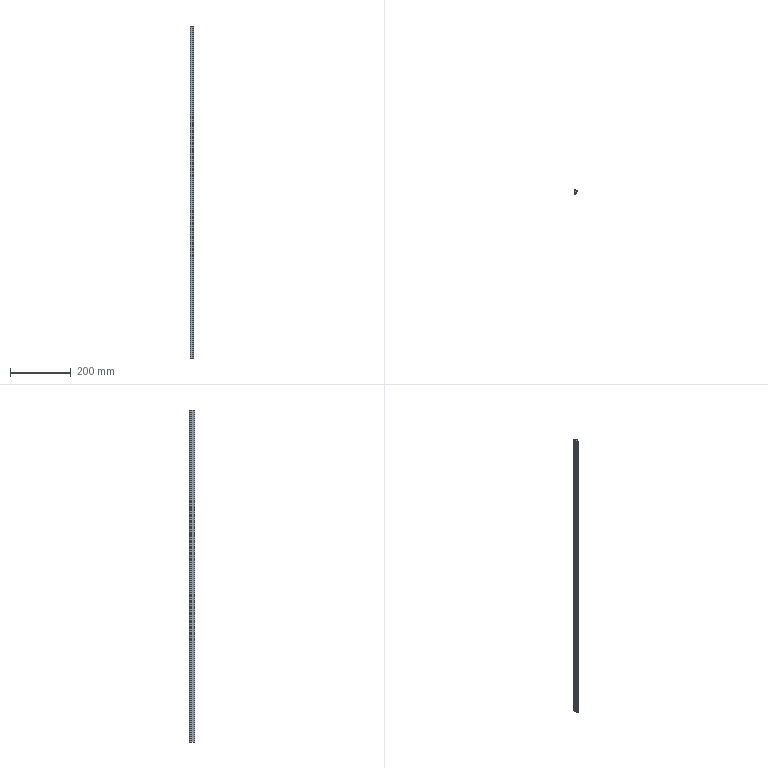Part | SolidWorks | features BaseBody 1, MoveFace 1 | 1 solid | 20 faces | box 10.8 x 17.5 x 1090 mm | volume 85893 mm3 | cylinder 11 | plane 9 | commonest cylinder face diameters 1.6 x2 14 x2 0.4 x1 0.6 x1 0.8 x1 2.6 x1
STEP:
#1=CARTESIAN_POINT('',(-3.236,-11.055,990.));
#2=VERTEX_POINT('',#1);
#3=CARTESIAN_POINT('',(-4.3,-10.3,990.));
#4=VERTEX_POINT('',#3);
#5=CARTESIAN_POINT('',(-3.5,-10.3,990.));
#6=DIRECTION('',(0.,0.,-1.));
#7=DIRECTION('',(1.,0.,0.));
#8=AXIS2_PLACEMENT_3D('',#5,#6,#7);
#9=CIRCLE('',#8,0.8);
#10=EDGE_CURVE('',#2,#4,#9,.T.);
#11=ORIENTED_EDGE('',*,*,#10,.T.);
#12=CARTESIAN_POINT('',(-4.3,-10.3,-100.));
#13=VERTEX_POINT('',#12);
#14=CARTESIAN_POINT('',(-4.3,-10.3,-100.));
#15=DIRECTION('',(0.,0.,-1.));
#16=VECTOR('',#15,1000.);
#17=LINE('',#14,#16);
#18=EDGE_CURVE('',#4,#13,#17,.T.);
#19=ORIENTED_EDGE('',*,*,#18,.T.);
#20=CARTESIAN_POINT('',(-3.236,-11.055,-100.));
#21=VERTEX_POINT('',#20);
#22=CARTESIAN_POINT('',(-3.5,-10.3,-100.));
#23=DIRECTION('',(0.,0.,1.));
#24=DIRECTION('',(-1.,0.,0.));
#25=AXIS2_PLACEMENT_3D('',#22,#23,#24);
#26=CIRCLE('',#25,0.8);
#27=EDGE_CURVE('',#13,#21,#26,.T.);
#28=ORIENTED_EDGE('',*,*,#27,.T.);
#29=CARTESIAN_POINT('',(-3.236,-11.055,-100.));
#30=DIRECTION('',(0.,0.,-1.));
#31=VECTOR('',#30,1000.);
#32=LINE('',#29,#31);
#33=EDGE_CURVE('',#2,#21,#32,.T.);
#34=ORIENTED_EDGE('',*,*,#33,.F.);
#35=EDGE_LOOP('',(#11,#19,#28,#34));
#36=FACE_OUTER_BOUND('',#35,.T.);
#37=CARTESIAN_POINT('',(-3.5,-10.3,-100.));
#38=DIRECTION('',(0.,0.,-1.));
#39=DIRECTION('',(-1.,0.,0.));
#40=AXIS2_PLACEMENT_3D('',#37,#38,#39);
#41=CYLINDRICAL_SURFACE('',#40,0.8);
#42=ADVANCED_FACE('',(#36),#41,.T.);
#43=CARTESIAN_POINT('',(1.184,-6.397,-100.));
#44=VERTEX_POINT('',#43);
#45=CARTESIAN_POINT('',(-5.702,-4.29,-100.));
#46=DIRECTION('',(0.,0.,1.));
#47=DIRECTION('',(-1.,0.,0.));
#48=AXIS2_PLACEMENT_3D('',#45,#46,#47);
#49=CIRCLE('',#48,7.201);
#50=EDGE_CURVE('',#21,#44,#49,.T.);
#51=ORIENTED_EDGE('',*,*,#50,.T.);
#52=CARTESIAN_POINT('',(1.184,-6.397,990.));
#53=VERTEX_POINT('',#52);
#54=CARTESIAN_POINT('',(1.184,-6.397,-100.));
#55=DIRECTION('',(0.,0.,1.));
#56=VECTOR('',#55,1000.);
#57=LINE('',#54,#56);
#58=EDGE_CURVE('',#44,#53,#57,.T.);
#59=ORIENTED_EDGE('',*,*,#58,.T.);
#60=CARTESIAN_POINT('',(-5.702,-4.29,990.));
#61=DIRECTION('',(0.,0.,-1.));
#62=DIRECTION('',(1.,0.,0.));
#63=AXIS2_PLACEMENT_3D('',#60,#61,#62);
#64=CIRCLE('',#63,7.201);
#65=EDGE_CURVE('',#53,#2,#64,.T.);
#66=ORIENTED_EDGE('',*,*,#65,.T.);
#67=ORIENTED_EDGE('',*,*,#33,.T.);
#68=EDGE_LOOP('',(#51,#59,#66,#67));
#69=FACE_OUTER_BOUND('',#68,.T.);
#70=CARTESIAN_POINT('',(-5.702,-4.29,-100.));
#71=DIRECTION('',(0.,0.,-1.));
#72=DIRECTION('',(-1.,0.,0.));
#73=AXIS2_PLACEMENT_3D('',#70,#71,#72);
#74=CYLINDRICAL_SURFACE('',#73,7.201);
#75=ADVANCED_FACE('',(#69),#74,.T.);
#76=CARTESIAN_POINT('',(0.9,-6.,-100.));
#77=VERTEX_POINT('',#76);
#78=CARTESIAN_POINT('',(0.9,-6.3,-100.));
#79=DIRECTION('',(0.,0.,1.));
#80=DIRECTION('',(-1.,0.,0.));
#81=AXIS2_PLACEMENT_3D('',#78,#79,#80);
#82=CIRCLE('',#81,0.3);
#83=EDGE_CURVE('',#44,#77,#82,.T.);
#84=ORIENTED_EDGE('',*,*,#83,.T.);
#85=CARTESIAN_POINT('',(0.9,-6.,990.));
#86=VERTEX_POINT('',#85);
#87=CARTESIAN_POINT('',(0.9,-6.,-100.));
#88=DIRECTION('',(0.,0.,1.));
#89=VECTOR('',#88,1000.);
#90=LINE('',#87,#89);
#91=EDGE_CURVE('',#77,#86,#90,.T.);
#92=ORIENTED_EDGE('',*,*,#91,.T.);
#93=CARTESIAN_POINT('',(0.9,-6.3,990.));
#94=DIRECTION('',(0.,0.,-1.));
#95=DIRECTION('',(1.,0.,0.));
#96=AXIS2_PLACEMENT_3D('',#93,#94,#95);
#97=CIRCLE('',#96,0.3);
#98=EDGE_CURVE('',#86,#53,#97,.T.);
#99=ORIENTED_EDGE('',*,*,#98,.T.);
#100=ORIENTED_EDGE('',*,*,#58,.F.);
#101=EDGE_LOOP('',(#84,#92,#99,#100));
#102=FACE_OUTER_BOUND('',#101,.T.);
#103=CARTESIAN_POINT('',(0.9,-6.3,-100.));
#104=DIRECTION('',(0.,0.,-1.));
#105=DIRECTION('',(-1.,0.,0.));
#106=AXIS2_PLACEMENT_3D('',#103,#104,#105);
#107=CYLINDRICAL_SURFACE('',#106,0.3);
#108=ADVANCED_FACE('',(#102),#107,.T.);
#109=CARTESIAN_POINT('',(-2.5,-0.5,-100.));
#110=VERTEX_POINT('',#109);
#111=CARTESIAN_POINT('',(-2.5,-6.153,-100.));
#112=VERTEX_POINT('',#111);
#113=CARTESIAN_POINT('',(-2.5,-6.397,-100.));
#114=DIRECTION('',(0.,-1.,0.));
#115=VECTOR('',#114,1000.);
#116=LINE('',#113,#115);
#117=EDGE_CURVE('',#110,#112,#116,.T.);
#118=ORIENTED_EDGE('',*,*,#117,.F.);
#119=CARTESIAN_POINT('',(-4.2,1.695,-100.));
#120=VERTEX_POINT('',#119);
#121=CARTESIAN_POINT('',(-1.701,1.875,-100.));
#122=DIRECTION('',(0.,0.,1.));
#123=DIRECTION('',(-1.,0.,0.));
#124=AXIS2_PLACEMENT_3D('',#121,#122,#123);
#125=CIRCLE('',#124,2.506);
#126=EDGE_CURVE('',#120,#110,#125,.T.);
#127=ORIENTED_EDGE('',*,*,#126,.F.);
#128=CARTESIAN_POINT('',(-4.2,5.1,-100.));
#129=VERTEX_POINT('',#128);
#130=CARTESIAN_POINT('',(-4.2,-6.397,-100.));
#131=DIRECTION('',(0.,-1.,0.));
#132=VECTOR('',#131,1000.);
#133=LINE('',#130,#132);
#134=EDGE_CURVE('',#129,#120,#133,.T.);
#135=ORIENTED_EDGE('',*,*,#134,.F.);
#136=CARTESIAN_POINT('',(-2.892,6.4,-100.));
#137=VERTEX_POINT('',#136);
#138=CARTESIAN_POINT('',(-2.9,5.1,-100.));
#139=DIRECTION('',(0.,0.,1.));
#140=DIRECTION('',(-1.,0.,0.));
#141=AXIS2_PLACEMENT_3D('',#138,#139,#140);
#142=CIRCLE('',#141,1.3);
#143=EDGE_CURVE('',#137,#129,#142,.T.);
#144=ORIENTED_EDGE('',*,*,#143,.F.);
#145=CARTESIAN_POINT('',(0.5,5.5,-100.));
#146=VERTEX_POINT('',#145);
#147=CARTESIAN_POINT('',(-2.934,-0.5999,-100.));
#148=DIRECTION('',(0.,0.,1.));
#149=DIRECTION('',(-1.,0.,0.));
#150=AXIS2_PLACEMENT_3D('',#147,#148,#149);
#151=CIRCLE('',#150,7.);
#152=EDGE_CURVE('',#146,#137,#151,.T.);
#153=ORIENTED_EDGE('',*,*,#152,.F.);
#154=CARTESIAN_POINT('',(5.5,1.7,-100.));
#155=VERTEX_POINT('',#154);
#156=CARTESIAN_POINT('',(5.5,1.7,-100.));
#157=DIRECTION('',(-0.7962,0.6051,0.));
#158=VECTOR('',#157,1000.);
#159=LINE('',#156,#158);
#160=EDGE_CURVE('',#155,#146,#159,.T.);
#161=ORIENTED_EDGE('',*,*,#160,.F.);
#162=CARTESIAN_POINT('',(6.458,-0.2215,-100.));
#163=VERTEX_POINT('',#162);
#164=CARTESIAN_POINT('',(6.458,-0.2215,-100.));
#165=DIRECTION('',(-0.4462,0.8949,0.));
#166=VECTOR('',#165,1000.);
#167=LINE('',#164,#166);
#168=EDGE_CURVE('',#163,#155,#167,.T.);
#169=ORIENTED_EDGE('',*,*,#168,.F.);
#170=CARTESIAN_POINT('',(5.895,-0.7433,-100.));
#171=VERTEX_POINT('',#170);
#172=CARTESIAN_POINT('',(6.1,-0.4,-100.));
#173=DIRECTION('',(0.,0.,1.));
#174=DIRECTION('',(-1.,0.,0.));
#175=AXIS2_PLACEMENT_3D('',#172,#173,#174);
#176=CIRCLE('',#175,0.4);
#177=EDGE_CURVE('',#171,#163,#176,.T.);
#178=ORIENTED_EDGE('',*,*,#177,.F.);
#179=CARTESIAN_POINT('',(3.,0.,-100.));
#180=VERTEX_POINT('',#179);
#181=CARTESIAN_POINT('',(2.746,-6.995,-100.));
#182=DIRECTION('',(0.,0.,-1.));
#183=DIRECTION('',(-1.,0.,0.));
#184=AXIS2_PLACEMENT_3D('',#181,#182,#183);
#185=CIRCLE('',#184,7.);
#186=EDGE_CURVE('',#180,#171,#185,.T.);
#187=ORIENTED_EDGE('',*,*,#186,.F.);
#188=CARTESIAN_POINT('',(0.,0.,-100.));
#189=VERTEX_POINT('',#188);
#190=CARTESIAN_POINT('',(-6.814,0.,-100.));
#191=DIRECTION('',(1.,0.,0.));
#192=VECTOR('',#191,1000.);
#193=LINE('',#190,#192);
#194=EDGE_CURVE('',#189,#180,#193,.T.);
#195=ORIENTED_EDGE('',*,*,#194,.F.);
#196=CARTESIAN_POINT('',(0.,-5.8,-100.));
#197=VERTEX_POINT('',#196);
#198=CARTESIAN_POINT('',(0.,-6.397,-100.));
#199=DIRECTION('',(0.,1.,0.));
#200=VECTOR('',#199,1000.);
#201=LINE('',#198,#200);
#202=EDGE_CURVE('',#197,#189,#201,.T.);
#203=ORIENTED_EDGE('',*,*,#202,.F.);
#204=CARTESIAN_POINT('',(0.2,-6.,-100.));
#205=VERTEX_POINT('',#204);
#206=CARTESIAN_POINT('',(0.2,-5.8,-100.));
#207=DIRECTION('',(0.,0.,1.));
#208=DIRECTION('',(-1.,0.,0.));
#209=AXIS2_PLACEMENT_3D('',#206,#207,#208);
#210=CIRCLE('',#209,0.2);
#211=EDGE_CURVE('',#197,#205,#210,.T.);
#212=ORIENTED_EDGE('',*,*,#211,.T.);
#213=CARTESIAN_POINT('',(-6.814,-6.,-100.));
#214=DIRECTION('',(-1.,0.,0.));
#215=VECTOR('',#214,1000.);
#216=LINE('',#213,#215);
#217=EDGE_CURVE('',#77,#205,#216,.T.);
#218=ORIENTED_EDGE('',*,*,#217,.F.);
#219=ORIENTED_EDGE('',*,*,#83,.F.);
#220=ORIENTED_EDGE('',*,*,#50,.F.);
#221=ORIENTED_EDGE('',*,*,#27,.F.);
#222=CARTESIAN_POINT('',(-3.998,-9.674,-100.));
#223=VERTEX_POINT('',#222);
#224=CARTESIAN_POINT('',(-3.5,-10.3,-100.));
#225=DIRECTION('',(0.,0.,1.));
#226=DIRECTION('',(-1.,0.,0.));
#227=AXIS2_PLACEMENT_3D('',#224,#225,#226);
#228=CIRCLE('',#227,0.8);
#229=EDGE_CURVE('',#223,#13,#228,.T.);
#230=ORIENTED_EDGE('',*,*,#229,.F.);
#231=CARTESIAN_POINT('',(-6.814,-6.397,-100.));
#232=DIRECTION('',(0.,0.,-1.));
#233=DIRECTION('',(-1.,0.,0.));
#234=AXIS2_PLACEMENT_3D('',#231,#232,#233);
#235=CIRCLE('',#234,4.321);
#236=EDGE_CURVE('',#112,#223,#235,.T.);
#237=ORIENTED_EDGE('',*,*,#236,.F.);
#238=EDGE_LOOP('',(#118,#127,#135,#144,#153,#161,#169,#178,#187,#195,#203,#212,#218,#219,#220,#221,#230,#237));
#239=FACE_OUTER_BOUND('',#238,.T.);
#240=CARTESIAN_POINT('',(-6.814,-6.397,-100.));
#241=DIRECTION('',(0.,0.,1.));
#242=DIRECTION('',(1.,0.,0.));
#243=AXIS2_PLACEMENT_3D('',#240,#241,#242);
#244=PLANE('',#243);
#245=ADVANCED_FACE('',(#239),#244,.F.);
#246=ORIENTED_EDGE('',*,*,#18,.F.);
#247=CARTESIAN_POINT('',(-3.998,-9.674,990.));
#248=VERTEX_POINT('',#247);
#249=CARTESIAN_POINT('',(-3.5,-10.3,990.));
#250=DIRECTION('',(0.,0.,-1.));
#251=DIRECTION('',(1.,0.,0.));
#252=AXIS2_PLACEMENT_3D('',#249,#250,#251);
#253=CIRCLE('',#252,0.8);
#254=EDGE_CURVE('',#4,#248,#253,.T.);
#255=ORIENTED_EDGE('',*,*,#254,.T.);
#256=CARTESIAN_POINT('',(-3.998,-9.674,-100.));
#257=DIRECTION('',(0.,0.,-1.));
#258=VECTOR('',#257,1000.);
#259=LINE('',#256,#258);
#260=EDGE_CURVE('',#248,#223,#259,.T.);
#261=ORIENTED_EDGE('',*,*,#260,.T.);
#262=ORIENTED_EDGE('',*,*,#229,.T.);
#263=EDGE_LOOP('',(#246,#255,#261,#262));
#264=FACE_OUTER_BOUND('',#263,.T.);
#265=CARTESIAN_POINT('',(-3.5,-10.3,-100.));
#266=DIRECTION('',(0.,0.,-1.));
#267=DIRECTION('',(-1.,0.,0.));
#268=AXIS2_PLACEMENT_3D('',#265,#266,#267);
#269=CYLINDRICAL_SURFACE('',#268,0.8);
#270=ADVANCED_FACE('',(#264),#269,.T.);
#271=CARTESIAN_POINT('',(-4.2,1.695,990.));
#272=VERTEX_POINT('',#271);
#273=CARTESIAN_POINT('',(-2.5,-0.5,990.));
#274=VERTEX_POINT('',#273);
#275=CARTESIAN_POINT('',(-1.701,1.875,990.));
#276=DIRECTION('',(0.,0.,1.));
#277=DIRECTION('',(1.,0.,0.));
#278=AXIS2_PLACEMENT_3D('',#275,#276,#277);
#279=CIRCLE('',#278,2.506);
#280=EDGE_CURVE('',#272,#274,#279,.T.);
#281=ORIENTED_EDGE('',*,*,#280,.T.);
#282=CARTESIAN_POINT('',(-2.5,-6.153,990.));
#283=VERTEX_POINT('',#282);
#284=CARTESIAN_POINT('',(-2.5,-6.397,990.));
#285=DIRECTION('',(0.,-1.,0.));
#286=VECTOR('',#285,1000.);
#287=LINE('',#284,#286);
#288=EDGE_CURVE('',#274,#283,#287,.T.);
#289=ORIENTED_EDGE('',*,*,#288,.T.);
#290=CARTESIAN_POINT('',(-6.814,-6.397,990.));
#291=DIRECTION('',(0.,0.,-1.));
#292=DIRECTION('',(1.,0.,0.));
#293=AXIS2_PLACEMENT_3D('',#290,#291,#292);
#294=CIRCLE('',#293,4.321);
#295=EDGE_CURVE('',#283,#248,#294,.T.);
#296=ORIENTED_EDGE('',*,*,#295,.T.);
#297=ORIENTED_EDGE('',*,*,#254,.F.);
#298=ORIENTED_EDGE('',*,*,#10,.F.);
#299=ORIENTED_EDGE('',*,*,#65,.F.);
#300=ORIENTED_EDGE('',*,*,#98,.F.);
#301=CARTESIAN_POINT('',(0.2,-6.,990.));
#302=VERTEX_POINT('',#301);
#303=CARTESIAN_POINT('',(-6.814,-6.,990.));
#304=DIRECTION('',(-1.,0.,0.));
#305=VECTOR('',#304,1000.);
#306=LINE('',#303,#305);
#307=EDGE_CURVE('',#86,#302,#306,.T.);
#308=ORIENTED_EDGE('',*,*,#307,.T.);
#309=CARTESIAN_POINT('',(0.,-5.8,990.));
#310=VERTEX_POINT('',#309);
#311=CARTESIAN_POINT('',(0.2,-5.8,990.));
#312=DIRECTION('',(0.,0.,-1.));
#313=DIRECTION('',(1.,0.,0.));
#314=AXIS2_PLACEMENT_3D('',#311,#312,#313);
#315=CIRCLE('',#314,0.2);
#316=EDGE_CURVE('',#302,#310,#315,.T.);
#317=ORIENTED_EDGE('',*,*,#316,.T.);
#318=CARTESIAN_POINT('',(0.,0.,990.));
#319=VERTEX_POINT('',#318);
#320=CARTESIAN_POINT('',(0.,-6.397,990.));
#321=DIRECTION('',(0.,1.,0.));
#322=VECTOR('',#321,1000.);
#323=LINE('',#320,#322);
#324=EDGE_CURVE('',#310,#319,#323,.T.);
#325=ORIENTED_EDGE('',*,*,#324,.T.);
#326=CARTESIAN_POINT('',(3.,0.,990.));
#327=VERTEX_POINT('',#326);
#328=CARTESIAN_POINT('',(-6.814,0.,990.));
#329=DIRECTION('',(1.,0.,0.));
#330=VECTOR('',#329,1000.);
#331=LINE('',#328,#330);
#332=EDGE_CURVE('',#319,#327,#331,.T.);
#333=ORIENTED_EDGE('',*,*,#332,.T.);
#334=CARTESIAN_POINT('',(5.895,-0.7433,990.));
#335=VERTEX_POINT('',#334);
#336=CARTESIAN_POINT('',(2.746,-6.995,990.));
#337=DIRECTION('',(0.,0.,-1.));
#338=DIRECTION('',(1.,0.,0.));
#339=AXIS2_PLACEMENT_3D('',#336,#337,#338);
#340=CIRCLE('',#339,7.);
#341=EDGE_CURVE('',#327,#335,#340,.T.);
#342=ORIENTED_EDGE('',*,*,#341,.T.);
#343=CARTESIAN_POINT('',(6.458,-0.2215,990.));
#344=VERTEX_POINT('',#343);
#345=CARTESIAN_POINT('',(6.1,-0.4,990.));
#346=DIRECTION('',(0.,0.,-1.));
#347=DIRECTION('',(1.,0.,0.));
#348=AXIS2_PLACEMENT_3D('',#345,#346,#347);
#349=CIRCLE('',#348,0.4);
#350=EDGE_CURVE('',#344,#335,#349,.T.);
#351=ORIENTED_EDGE('',*,*,#350,.F.);
#352=CARTESIAN_POINT('',(5.5,1.7,990.));
#353=VERTEX_POINT('',#352);
#354=CARTESIAN_POINT('',(6.282,0.1323,990.));
#355=DIRECTION('',(-0.4462,0.8949,0.));
#356=VECTOR('',#355,1000.);
#357=LINE('',#354,#356);
#358=EDGE_CURVE('',#344,#353,#357,.T.);
#359=ORIENTED_EDGE('',*,*,#358,.T.);
#360=CARTESIAN_POINT('',(0.5,5.5,990.));
#361=VERTEX_POINT('',#360);
#362=CARTESIAN_POINT('',(1.595,4.668,990.));
#363=DIRECTION('',(-0.7962,0.6051,0.));
#364=VECTOR('',#363,1000.);
#365=LINE('',#362,#364);
#366=EDGE_CURVE('',#353,#361,#365,.T.);
#367=ORIENTED_EDGE('',*,*,#366,.T.);
#368=CARTESIAN_POINT('',(-2.892,6.4,990.));
#369=VERTEX_POINT('',#368);
#370=CARTESIAN_POINT('',(-2.934,-0.5999,990.));
#371=DIRECTION('',(0.,0.,1.));
#372=DIRECTION('',(1.,0.,0.));
#373=AXIS2_PLACEMENT_3D('',#370,#371,#372);
#374=CIRCLE('',#373,7.);
#375=EDGE_CURVE('',#361,#369,#374,.T.);
#376=ORIENTED_EDGE('',*,*,#375,.T.);
#377=CARTESIAN_POINT('',(-4.2,5.1,990.));
#378=VERTEX_POINT('',#377);
#379=CARTESIAN_POINT('',(-2.9,5.1,990.));
#380=DIRECTION('',(0.,0.,1.));
#381=DIRECTION('',(1.,0.,0.));
#382=AXIS2_PLACEMENT_3D('',#379,#380,#381);
#383=CIRCLE('',#382,1.3);
#384=EDGE_CURVE('',#369,#378,#383,.T.);
#385=ORIENTED_EDGE('',*,*,#384,.T.);
#386=CARTESIAN_POINT('',(-4.2,-6.397,990.));
#387=DIRECTION('',(0.,-1.,0.));
#388=VECTOR('',#387,1000.);
#389=LINE('',#386,#388);
#390=EDGE_CURVE('',#378,#272,#389,.T.);
#391=ORIENTED_EDGE('',*,*,#390,.T.);
#392=EDGE_LOOP('',(#281,#289,#296,#297,#298,#299,#300,#308,#317,#325,#333,#342,#351,#359,#367,#376,#385,#391));
#393=FACE_OUTER_BOUND('',#392,.T.);
#394=CARTESIAN_POINT('',(-6.814,-6.397,990.));
#395=DIRECTION('',(0.,0.,1.));
#396=DIRECTION('',(1.,0.,0.));
#397=AXIS2_PLACEMENT_3D('',#394,#395,#396);
#398=PLANE('',#397);
#399=ADVANCED_FACE('',(#393),#398,.T.);
#400=ORIENTED_EDGE('',*,*,#217,.T.);
#401=CARTESIAN_POINT('',(0.2,-6.,-100.));
#402=DIRECTION('',(0.,0.,1.));
#403=VECTOR('',#402,1000.);
#404=LINE('',#401,#403);
#405=EDGE_CURVE('',#205,#302,#404,.T.);
#406=ORIENTED_EDGE('',*,*,#405,.T.);
#407=ORIENTED_EDGE('',*,*,#307,.F.);
#408=ORIENTED_EDGE('',*,*,#91,.F.);
#409=EDGE_LOOP('',(#400,#406,#407,#408));
#410=FACE_OUTER_BOUND('',#409,.T.);
#411=CARTESIAN_POINT('',(0.9,-6.,-100.));
#412=DIRECTION('',(0.,1.,0.));
#413=DIRECTION('',(0.,0.,1.));
#414=AXIS2_PLACEMENT_3D('',#411,#412,#413);
#415=PLANE('',#414);
#416=ADVANCED_FACE('',(#410),#415,.T.);
#417=CARTESIAN_POINT('',(-2.5,-6.153,-100.));
#418=DIRECTION('',(0.,0.,1.));
#419=VECTOR('',#418,1000.);
#420=LINE('',#417,#419);
#421=EDGE_CURVE('',#112,#283,#420,.T.);
#422=ORIENTED_EDGE('',*,*,#421,.F.);
#423=ORIENTED_EDGE('',*,*,#236,.T.);
#424=ORIENTED_EDGE('',*,*,#260,.F.);
#425=ORIENTED_EDGE('',*,*,#295,.F.);
#426=EDGE_LOOP('',(#422,#423,#424,#425));
#427=FACE_OUTER_BOUND('',#426,.T.);
#428=CARTESIAN_POINT('',(-6.814,-6.397,-100.));
#429=DIRECTION('',(0.,0.,-1.));
#430=DIRECTION('',(-1.,0.,0.));
#431=AXIS2_PLACEMENT_3D('',#428,#429,#430);
#432=CYLINDRICAL_SURFACE('',#431,4.321);
#433=ADVANCED_FACE('',(#427),#432,.F.);
#434=ORIENTED_EDGE('',*,*,#117,.T.);
#435=ORIENTED_EDGE('',*,*,#421,.T.);
#436=ORIENTED_EDGE('',*,*,#288,.F.);
#437=CARTESIAN_POINT('',(-2.5,-0.5,-100.));
#438=DIRECTION('',(0.,0.,-1.));
#439=VECTOR('',#438,1000.);
#440=LINE('',#437,#439);
#441=EDGE_CURVE('',#274,#110,#440,.T.);
#442=ORIENTED_EDGE('',*,*,#441,.T.);
#443=EDGE_LOOP('',(#434,#435,#436,#442));
#444=FACE_OUTER_BOUND('',#443,.T.);
#445=CARTESIAN_POINT('',(-2.5,-0.5,-100.));
#446=DIRECTION('',(-1.,0.,0.));
#447=DIRECTION('',(0.,0.,1.));
#448=AXIS2_PLACEMENT_3D('',#445,#446,#447);
#449=PLANE('',#448);
#450=ADVANCED_FACE('',(#444),#449,.T.);
#451=ORIENTED_EDGE('',*,*,#126,.T.);
#452=ORIENTED_EDGE('',*,*,#441,.F.);
#453=ORIENTED_EDGE('',*,*,#280,.F.);
#454=CARTESIAN_POINT('',(-4.2,1.695,-100.));
#455=DIRECTION('',(0.,0.,-1.));
#456=VECTOR('',#455,1000.);
#457=LINE('',#454,#456);
#458=EDGE_CURVE('',#272,#120,#457,.T.);
#459=ORIENTED_EDGE('',*,*,#458,.T.);
#460=EDGE_LOOP('',(#451,#452,#453,#459));
#461=FACE_OUTER_BOUND('',#460,.T.);
#462=CARTESIAN_POINT('',(-1.701,1.875,-100.));
#463=DIRECTION('',(0.,0.,-1.));
#464=DIRECTION('',(-1.,0.,0.));
#465=AXIS2_PLACEMENT_3D('',#462,#463,#464);
#466=CYLINDRICAL_SURFACE('',#465,2.506);
#467=ADVANCED_FACE('',(#461),#466,.T.);
#468=ORIENTED_EDGE('',*,*,#134,.T.);
#469=ORIENTED_EDGE('',*,*,#458,.F.);
#470=ORIENTED_EDGE('',*,*,#390,.F.);
#471=CARTESIAN_POINT('',(-4.2,5.1,-100.));
#472=DIRECTION('',(0.,0.,-1.));
#473=VECTOR('',#472,1000.);
#474=LINE('',#471,#473);
#475=EDGE_CURVE('',#378,#129,#474,.T.);
#476=ORIENTED_EDGE('',*,*,#475,.T.);
#477=EDGE_LOOP('',(#468,#469,#470,#476));
#478=FACE_OUTER_BOUND('',#477,.T.);
#479=CARTESIAN_POINT('',(-4.2,5.1,-100.));
#480=DIRECTION('',(-1.,0.,0.));
#481=DIRECTION('',(0.,0.,1.));
#482=AXIS2_PLACEMENT_3D('',#479,#480,#481);
#483=PLANE('',#482);
#484=ADVANCED_FACE('',(#478),#483,.T.);
#485=ORIENTED_EDGE('',*,*,#143,.T.);
#486=ORIENTED_EDGE('',*,*,#475,.F.);
#487=ORIENTED_EDGE('',*,*,#384,.F.);
#488=CARTESIAN_POINT('',(-2.892,6.4,-100.));
#489=DIRECTION('',(0.,0.,-1.));
#490=VECTOR('',#489,1000.);
#491=LINE('',#488,#490);
#492=EDGE_CURVE('',#369,#137,#491,.T.);
#493=ORIENTED_EDGE('',*,*,#492,.T.);
#494=EDGE_LOOP('',(#485,#486,#487,#493));
#495=FACE_OUTER_BOUND('',#494,.T.);
#496=CARTESIAN_POINT('',(-2.9,5.1,-100.));
#497=DIRECTION('',(0.,0.,-1.));
#498=DIRECTION('',(-1.,0.,0.));
#499=AXIS2_PLACEMENT_3D('',#496,#497,#498);
#500=CYLINDRICAL_SURFACE('',#499,1.3);
#501=ADVANCED_FACE('',(#495),#500,.T.);
#502=ORIENTED_EDGE('',*,*,#152,.T.);
#503=ORIENTED_EDGE('',*,*,#492,.F.);
#504=ORIENTED_EDGE('',*,*,#375,.F.);
#505=CARTESIAN_POINT('',(0.5,5.5,-100.));
#506=DIRECTION('',(0.,0.,-1.));
#507=VECTOR('',#506,1000.);
#508=LINE('',#505,#507);
#509=EDGE_CURVE('',#361,#146,#508,.T.);
#510=ORIENTED_EDGE('',*,*,#509,.T.);
#511=EDGE_LOOP('',(#502,#503,#504,#510));
#512=FACE_OUTER_BOUND('',#511,.T.);
#513=CARTESIAN_POINT('',(-2.934,-0.5999,-100.));
#514=DIRECTION('',(0.,0.,-1.));
#515=DIRECTION('',(-1.,0.,0.));
#516=AXIS2_PLACEMENT_3D('',#513,#514,#515);
#517=CYLINDRICAL_SURFACE('',#516,7.);
#518=ADVANCED_FACE('',(#512),#517,.T.);
#519=ORIENTED_EDGE('',*,*,#160,.T.);
#520=ORIENTED_EDGE('',*,*,#509,.F.);
#521=ORIENTED_EDGE('',*,*,#366,.F.);
#522=CARTESIAN_POINT('',(5.5,1.7,-100.));
#523=DIRECTION('',(0.,0.,-1.));
#524=VECTOR('',#523,1000.);
#525=LINE('',#522,#524);
#526=EDGE_CURVE('',#353,#155,#525,.T.);
#527=ORIENTED_EDGE('',*,*,#526,.T.);
#528=EDGE_LOOP('',(#519,#520,#521,#527));
#529=FACE_OUTER_BOUND('',#528,.T.);
#530=CARTESIAN_POINT('',(5.5,1.7,-100.));
#531=DIRECTION('',(0.6051,0.7962,0.));
#532=DIRECTION('',(-0.7962,0.6051,0.));
#533=AXIS2_PLACEMENT_3D('',#530,#531,#532);
#534=PLANE('',#533);
#535=ADVANCED_FACE('',(#529),#534,.T.);
#536=ORIENTED_EDGE('',*,*,#168,.T.);
#537=ORIENTED_EDGE('',*,*,#526,.F.);
#538=ORIENTED_EDGE('',*,*,#358,.F.);
#539=CARTESIAN_POINT('',(6.458,-0.2215,-100.));
#540=DIRECTION('',(0.,0.,-1.));
#541=VECTOR('',#540,1000.);
#542=LINE('',#539,#541);
#543=EDGE_CURVE('',#344,#163,#542,.T.);
#544=ORIENTED_EDGE('',*,*,#543,.T.);
#545=EDGE_LOOP('',(#536,#537,#538,#544));
#546=FACE_OUTER_BOUND('',#545,.T.);
#547=CARTESIAN_POINT('',(6.458,-0.2215,-100.));
#548=DIRECTION('',(0.8949,0.4462,0.));
#549=DIRECTION('',(-0.4462,0.8949,0.));
#550=AXIS2_PLACEMENT_3D('',#547,#548,#549);
#551=PLANE('',#550);
#552=ADVANCED_FACE('',(#546),#551,.T.);
#553=CARTESIAN_POINT('',(3.,0.,-100.));
#554=DIRECTION('',(0.,0.,1.));
#555=VECTOR('',#554,1000.);
#556=LINE('',#553,#555);
#557=EDGE_CURVE('',#180,#327,#556,.T.);
#558=ORIENTED_EDGE('',*,*,#557,.F.);
#559=ORIENTED_EDGE('',*,*,#186,.T.);
#560=CARTESIAN_POINT('',(5.895,-0.7433,-100.));
#561=DIRECTION('',(0.,0.,-1.));
#562=VECTOR('',#561,1000.);
#563=LINE('',#560,#562);
#564=EDGE_CURVE('',#335,#171,#563,.T.);
#565=ORIENTED_EDGE('',*,*,#564,.F.);
#566=ORIENTED_EDGE('',*,*,#341,.F.);
#567=EDGE_LOOP('',(#558,#559,#565,#566));
#568=FACE_OUTER_BOUND('',#567,.T.);
#569=CARTESIAN_POINT('',(2.746,-6.995,-100.));
#570=DIRECTION('',(0.,0.,-1.));
#571=DIRECTION('',(-1.,0.,0.));
#572=AXIS2_PLACEMENT_3D('',#569,#570,#571);
#573=CYLINDRICAL_SURFACE('',#572,7.);
#574=ADVANCED_FACE('',(#568),#573,.F.);
#575=ORIENTED_EDGE('',*,*,#194,.T.);
#576=ORIENTED_EDGE('',*,*,#557,.T.);
#577=ORIENTED_EDGE('',*,*,#332,.F.);
#578=CARTESIAN_POINT('',(0.,0.,-100.));
#579=DIRECTION('',(0.,0.,-1.));
#580=VECTOR('',#579,1000.);
#581=LINE('',#578,#580);
#582=EDGE_CURVE('',#319,#189,#581,.T.);
#583=ORIENTED_EDGE('',*,*,#582,.T.);
#584=EDGE_LOOP('',(#575,#576,#577,#583));
#585=FACE_OUTER_BOUND('',#584,.T.);
#586=CARTESIAN_POINT('',(0.,0.,-100.));
#587=DIRECTION('',(0.,-1.,0.));
#588=DIRECTION('',(0.,0.,-1.));
#589=AXIS2_PLACEMENT_3D('',#586,#587,#588);
#590=PLANE('',#589);
#591=ADVANCED_FACE('',(#585),#590,.T.);
#592=ORIENTED_EDGE('',*,*,#202,.T.);
#593=ORIENTED_EDGE('',*,*,#582,.F.);
#594=ORIENTED_EDGE('',*,*,#324,.F.);
#595=CARTESIAN_POINT('',(0.,-5.8,-100.));
#596=DIRECTION('',(0.,0.,-1.));
#597=VECTOR('',#596,1000.);
#598=LINE('',#595,#597);
#599=EDGE_CURVE('',#310,#197,#598,.T.);
#600=ORIENTED_EDGE('',*,*,#599,.T.);
#601=EDGE_LOOP('',(#592,#593,#594,#600));
#602=FACE_OUTER_BOUND('',#601,.T.);
#603=CARTESIAN_POINT('',(0.,-5.8,-100.));
#604=DIRECTION('',(1.,0.,0.));
#605=DIRECTION('',(0.,0.,-1.));
#606=AXIS2_PLACEMENT_3D('',#603,#604,#605);
#607=PLANE('',#606);
#608=ADVANCED_FACE('',(#602),#607,.T.);
#609=ORIENTED_EDGE('',*,*,#405,.F.);
#610=ORIENTED_EDGE('',*,*,#211,.F.);
#611=ORIENTED_EDGE('',*,*,#599,.F.);
#612=ORIENTED_EDGE('',*,*,#316,.F.);
#613=EDGE_LOOP('',(#609,#610,#611,#612));
#614=FACE_OUTER_BOUND('',#613,.T.);
#615=CARTESIAN_POINT('',(0.2,-5.8,-100.));
#616=DIRECTION('',(0.,0.,-1.));
#617=DIRECTION('',(-1.,0.,0.));
#618=AXIS2_PLACEMENT_3D('',#615,#616,#617);
#619=CYLINDRICAL_SURFACE('',#618,0.2);
#620=ADVANCED_FACE('',(#614),#619,.F.);
#621=ORIENTED_EDGE('',*,*,#177,.T.);
#622=ORIENTED_EDGE('',*,*,#543,.F.);
#623=ORIENTED_EDGE('',*,*,#350,.T.);
#624=ORIENTED_EDGE('',*,*,#564,.T.);
#625=EDGE_LOOP('',(#621,#622,#623,#624));
#626=FACE_OUTER_BOUND('',#625,.T.);
#627=CARTESIAN_POINT('',(6.1,-0.4,-100.));
#628=DIRECTION('',(0.,0.,-1.));
#629=DIRECTION('',(-1.,0.,0.));
#630=AXIS2_PLACEMENT_3D('',#627,#628,#629);
#631=CYLINDRICAL_SURFACE('',#630,0.4);
#632=ADVANCED_FACE('',(#626),#631,.T.);
#633=CLOSED_SHELL('',(#42,#75,#108,#245,#270,#399,#416,#433,#450,#467,#484,#501,#518,#535,#552,#574,#591,#608,#620,#632));
#634=MANIFOLD_SOLID_BREP('',#633);
#635=CARTESIAN_POINT('',(0.,0.,0.));
#636=DIRECTION('',(0.,0.,1.));
#637=DIRECTION('',(1.,0.,0.));
#638=AXIS2_PLACEMENT_3D('',#635,#636,#637);
#639=(LENGTH_UNIT()NAMED_UNIT(*)SI_UNIT(.MILLI.,.METRE.));
#640=UNCERTAINTY_MEASURE_WITH_UNIT(LENGTH_MEASURE(0.00001),#639,'','');
#641=(NAMED_UNIT(*)PLANE_ANGLE_UNIT()SI_UNIT($,.RADIAN.));
#642=(NAMED_UNIT(*)SI_UNIT($,.STERADIAN.)SOLID_ANGLE_UNIT());
#643=(GEOMETRIC_REPRESENTATION_CONTEXT(3)GLOBAL_UNCERTAINTY_ASSIGNED_CONTEXT((#640))GLOBAL_UNIT_ASSIGNED_CONTEXT((#639,#641,#642))REPRESENTATION_CONTEXT('',''));
#644=ADVANCED_BREP_SHAPE_REPRESENTATION('',(#634,#638),#643);